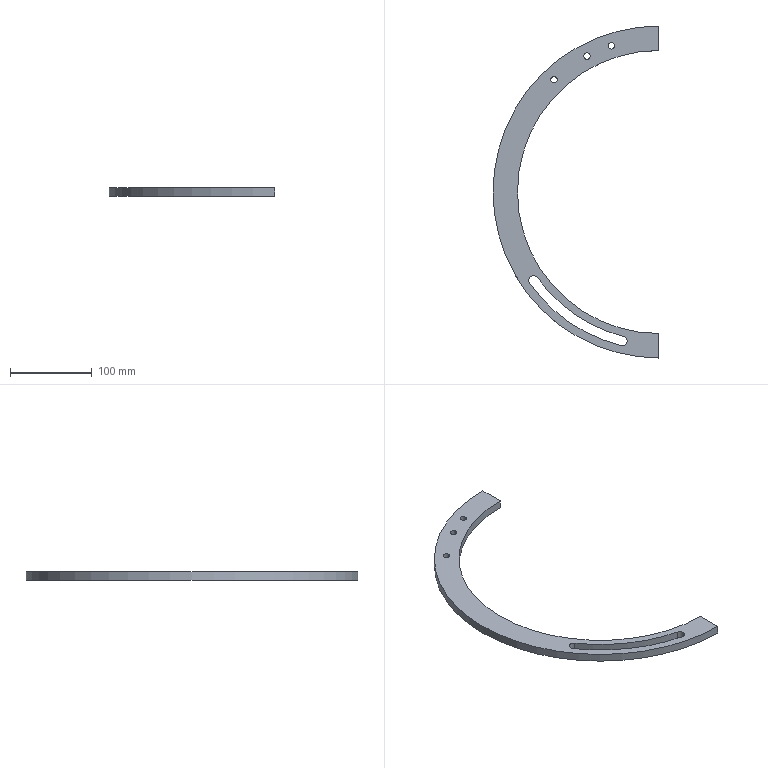Part | SolidWorks | features Cut 3, Extrusion 1 | 1 solid | 17 faces | box 203.295 x 406.59 x 10 mm | volume 159222 mm3 | cylinder 13 | plane 4 | commonest cylinder face diameters 8 x6 11.641 x3 346.59 x1 364.161 x1 387.442 x1 406.59 x1
STEP:
#1=CARTESIAN_POINT('',(166.898,320.188,0.));
#2=VERTEX_POINT('',#1);
#3=CARTESIAN_POINT('',(158.898,320.188,0.));
#4=VERTEX_POINT('',#3);
#5=CARTESIAN_POINT('',(162.898,320.188,0.));
#6=DIRECTION('',(0.,0.,-1.));
#7=DIRECTION('',(-1.,0.,0.));
#8=AXIS2_PLACEMENT_3D('',#5,#6,#7);
#9=CIRCLE('',#8,4.);
#10=EDGE_CURVE('',#2,#4,#9,.T.);
#11=ORIENTED_EDGE('',*,*,#10,.F.);
#12=CARTESIAN_POINT('',(166.898,320.188,-10.));
#13=VERTEX_POINT('',#12);
#14=CARTESIAN_POINT('',(166.898,320.188,0.));
#15=DIRECTION('',(0.,0.,-1.));
#16=VECTOR('',#15,1000.);
#17=LINE('',#14,#16);
#18=EDGE_CURVE('',#2,#13,#17,.T.);
#19=ORIENTED_EDGE('',*,*,#18,.T.);
#20=CARTESIAN_POINT('',(158.898,320.188,-10.));
#21=VERTEX_POINT('',#20);
#22=CARTESIAN_POINT('',(162.898,320.188,-10.));
#23=DIRECTION('',(0.,0.,1.));
#24=DIRECTION('',(1.,0.,0.));
#25=AXIS2_PLACEMENT_3D('',#22,#23,#24);
#26=CIRCLE('',#25,4.);
#27=EDGE_CURVE('',#21,#13,#26,.T.);
#28=ORIENTED_EDGE('',*,*,#27,.F.);
#29=CARTESIAN_POINT('',(158.898,320.188,0.));
#30=DIRECTION('',(0.,0.,-1.));
#31=VECTOR('',#30,1000.);
#32=LINE('',#29,#31);
#33=EDGE_CURVE('',#4,#21,#32,.T.);
#34=ORIENTED_EDGE('',*,*,#33,.F.);
#35=EDGE_LOOP('',(#11,#19,#28,#34));
#36=FACE_OUTER_BOUND('',#35,.T.);
#37=CARTESIAN_POINT('',(162.898,320.188,0.));
#38=DIRECTION('',(0.,0.,-1.));
#39=DIRECTION('',(-1.,0.,0.));
#40=AXIS2_PLACEMENT_3D('',#37,#38,#39);
#41=CYLINDRICAL_SURFACE('',#40,4.);
#42=ADVANCED_FACE('',(#36),#41,.F.);
#43=CARTESIAN_POINT('',(237.318,361.783,0.));
#44=VERTEX_POINT('',#43);
#45=CARTESIAN_POINT('',(229.318,361.783,0.));
#46=VERTEX_POINT('',#45);
#47=CARTESIAN_POINT('',(233.318,361.783,0.));
#48=DIRECTION('',(0.,0.,-1.));
#49=DIRECTION('',(-1.,0.,0.));
#50=AXIS2_PLACEMENT_3D('',#47,#48,#49);
#51=CIRCLE('',#50,4.);
#52=EDGE_CURVE('',#44,#46,#51,.T.);
#53=ORIENTED_EDGE('',*,*,#52,.F.);
#54=CARTESIAN_POINT('',(237.318,361.783,-10.));
#55=VERTEX_POINT('',#54);
#56=CARTESIAN_POINT('',(237.318,361.783,0.));
#57=DIRECTION('',(0.,0.,-1.));
#58=VECTOR('',#57,1000.);
#59=LINE('',#56,#58);
#60=EDGE_CURVE('',#44,#55,#59,.T.);
#61=ORIENTED_EDGE('',*,*,#60,.T.);
#62=CARTESIAN_POINT('',(229.318,361.783,-10.));
#63=VERTEX_POINT('',#62);
#64=CARTESIAN_POINT('',(233.318,361.783,-10.));
#65=DIRECTION('',(0.,0.,1.));
#66=DIRECTION('',(1.,0.,0.));
#67=AXIS2_PLACEMENT_3D('',#64,#65,#66);
#68=CIRCLE('',#67,4.);
#69=EDGE_CURVE('',#63,#55,#68,.T.);
#70=ORIENTED_EDGE('',*,*,#69,.F.);
#71=CARTESIAN_POINT('',(229.318,361.783,0.));
#72=DIRECTION('',(0.,0.,-1.));
#73=VECTOR('',#72,1000.);
#74=LINE('',#71,#73);
#75=EDGE_CURVE('',#46,#63,#74,.T.);
#76=ORIENTED_EDGE('',*,*,#75,.F.);
#77=EDGE_LOOP('',(#53,#61,#70,#76));
#78=FACE_OUTER_BOUND('',#77,.T.);
#79=CARTESIAN_POINT('',(233.318,361.783,0.));
#80=DIRECTION('',(0.,0.,-1.));
#81=DIRECTION('',(-1.,0.,0.));
#82=AXIS2_PLACEMENT_3D('',#79,#80,#81);
#83=CYLINDRICAL_SURFACE('',#82,4.);
#84=ADVANCED_FACE('',(#78),#83,.F.);
#85=CARTESIAN_POINT('',(207.412,349.105,0.));
#86=VERTEX_POINT('',#85);
#87=CARTESIAN_POINT('',(199.412,349.105,0.));
#88=VERTEX_POINT('',#87);
#89=CARTESIAN_POINT('',(203.412,349.105,0.));
#90=DIRECTION('',(0.,0.,-1.));
#91=DIRECTION('',(-1.,0.,0.));
#92=AXIS2_PLACEMENT_3D('',#89,#90,#91);
#93=CIRCLE('',#92,4.);
#94=EDGE_CURVE('',#86,#88,#93,.T.);
#95=ORIENTED_EDGE('',*,*,#94,.F.);
#96=CARTESIAN_POINT('',(207.412,349.105,-10.));
#97=VERTEX_POINT('',#96);
#98=CARTESIAN_POINT('',(207.412,349.105,0.));
#99=DIRECTION('',(0.,0.,-1.));
#100=VECTOR('',#99,1000.);
#101=LINE('',#98,#100);
#102=EDGE_CURVE('',#86,#97,#101,.T.);
#103=ORIENTED_EDGE('',*,*,#102,.T.);
#104=CARTESIAN_POINT('',(199.412,349.105,-10.));
#105=VERTEX_POINT('',#104);
#106=CARTESIAN_POINT('',(203.412,349.105,-10.));
#107=DIRECTION('',(0.,0.,1.));
#108=DIRECTION('',(1.,0.,0.));
#109=AXIS2_PLACEMENT_3D('',#106,#107,#108);
#110=CIRCLE('',#109,4.);
#111=EDGE_CURVE('',#105,#97,#110,.T.);
#112=ORIENTED_EDGE('',*,*,#111,.F.);
#113=CARTESIAN_POINT('',(199.412,349.105,0.));
#114=DIRECTION('',(0.,0.,-1.));
#115=VECTOR('',#114,1000.);
#116=LINE('',#113,#115);
#117=EDGE_CURVE('',#88,#105,#116,.T.);
#118=ORIENTED_EDGE('',*,*,#117,.F.);
#119=EDGE_LOOP('',(#95,#103,#112,#118));
#120=FACE_OUTER_BOUND('',#119,.T.);
#121=CARTESIAN_POINT('',(203.412,349.105,0.));
#122=DIRECTION('',(0.,0.,-1.));
#123=DIRECTION('',(-1.,0.,0.));
#124=AXIS2_PLACEMENT_3D('',#121,#122,#123);
#125=CYLINDRICAL_SURFACE('',#124,4.);
#126=ADVANCED_FACE('',(#120),#125,.F.);
#127=CARTESIAN_POINT('',(142.762,77.826,0.));
#128=VERTEX_POINT('',#127);
#129=CARTESIAN_POINT('',(132.185,74.473,0.));
#130=VERTEX_POINT('',#129);
#131=CARTESIAN_POINT('',(138.005,74.473,0.));
#132=DIRECTION('',(0.,0.,1.));
#133=DIRECTION('',(1.,0.,0.));
#134=AXIS2_PLACEMENT_3D('',#131,#132,#133);
#135=CIRCLE('',#134,5.82);
#136=EDGE_CURVE('',#128,#130,#135,.T.);
#137=ORIENTED_EDGE('',*,*,#136,.T.);
#138=CARTESIAN_POINT('',(132.185,74.473,-10.));
#139=VERTEX_POINT('',#138);
#140=CARTESIAN_POINT('',(132.185,74.473,175.));
#141=DIRECTION('',(0.,0.,-1.));
#142=VECTOR('',#141,1000.);
#143=LINE('',#140,#142);
#144=EDGE_CURVE('',#130,#139,#143,.T.);
#145=ORIENTED_EDGE('',*,*,#144,.T.);
#146=CARTESIAN_POINT('',(142.762,77.826,-10.));
#147=VERTEX_POINT('',#146);
#148=CARTESIAN_POINT('',(138.005,74.473,-10.));
#149=DIRECTION('',(0.,0.,-1.));
#150=DIRECTION('',(-1.,0.,0.));
#151=AXIS2_PLACEMENT_3D('',#148,#149,#150);
#152=CIRCLE('',#151,5.82);
#153=EDGE_CURVE('',#139,#147,#152,.T.);
#154=ORIENTED_EDGE('',*,*,#153,.T.);
#155=CARTESIAN_POINT('',(142.762,77.826,175.));
#156=DIRECTION('',(0.,0.,-1.));
#157=VECTOR('',#156,1000.);
#158=LINE('',#155,#157);
#159=EDGE_CURVE('',#128,#147,#158,.T.);
#160=ORIENTED_EDGE('',*,*,#159,.F.);
#161=EDGE_LOOP('',(#137,#145,#154,#160));
#162=FACE_OUTER_BOUND('',#161,.T.);
#163=CARTESIAN_POINT('',(138.005,74.473,175.));
#164=DIRECTION('',(0.,0.,-1.));
#165=DIRECTION('',(-1.,0.,0.));
#166=AXIS2_PLACEMENT_3D('',#163,#164,#165);
#167=CYLINDRICAL_SURFACE('',#166,5.82);
#168=ADVANCED_FACE('',(#162),#167,.F.);
#169=CARTESIAN_POINT('',(291.585,-20.564,0.));
#170=VERTEX_POINT('',#169);
#171=CARTESIAN_POINT('',(291.585,-20.564,-10.));
#172=VERTEX_POINT('',#171);
#173=CARTESIAN_POINT('',(291.585,-20.564,-10.));
#174=DIRECTION('',(0.,0.,-1.));
#175=VECTOR('',#174,1000.);
#176=LINE('',#173,#175);
#177=EDGE_CURVE('',#170,#172,#176,.T.);
#178=ORIENTED_EDGE('',*,*,#177,.F.);
#179=CARTESIAN_POINT('',(291.585,386.026,0.));
#180=VERTEX_POINT('',#179);
#181=CARTESIAN_POINT('',(291.585,182.731,0.));
#182=DIRECTION('',(0.,0.,1.));
#183=DIRECTION('',(1.,0.,0.));
#184=AXIS2_PLACEMENT_3D('',#181,#182,#183);
#185=CIRCLE('',#184,203.295);
#186=EDGE_CURVE('',#180,#170,#185,.T.);
#187=ORIENTED_EDGE('',*,*,#186,.F.);
#188=CARTESIAN_POINT('',(291.585,386.026,-10.));
#189=VERTEX_POINT('',#188);
#190=CARTESIAN_POINT('',(291.585,386.026,-10.));
#191=DIRECTION('',(0.,0.,1.));
#192=VECTOR('',#191,1000.);
#193=LINE('',#190,#192);
#194=EDGE_CURVE('',#189,#180,#193,.T.);
#195=ORIENTED_EDGE('',*,*,#194,.F.);
#196=CARTESIAN_POINT('',(291.585,182.731,-10.));
#197=DIRECTION('',(0.,0.,1.));
#198=DIRECTION('',(1.,0.,0.));
#199=AXIS2_PLACEMENT_3D('',#196,#197,#198);
#200=CIRCLE('',#199,203.295);
#201=EDGE_CURVE('',#189,#172,#200,.T.);
#202=ORIENTED_EDGE('',*,*,#201,.T.);
#203=EDGE_LOOP('',(#178,#187,#195,#202));
#204=FACE_OUTER_BOUND('',#203,.T.);
#205=CARTESIAN_POINT('',(291.585,182.731,-10.));
#206=DIRECTION('',(0.,0.,1.));
#207=DIRECTION('',(1.,0.,0.));
#208=AXIS2_PLACEMENT_3D('',#205,#206,#207);
#209=CYLINDRICAL_SURFACE('',#208,203.295);
#210=ADVANCED_FACE('',(#204),#209,.T.);
#211=ORIENTED_EDGE('',*,*,#27,.T.);
#212=CARTESIAN_POINT('',(162.898,320.188,-10.));
#213=DIRECTION('',(0.,0.,1.));
#214=DIRECTION('',(1.,0.,0.));
#215=AXIS2_PLACEMENT_3D('',#212,#213,#214);
#216=CIRCLE('',#215,4.);
#217=EDGE_CURVE('',#13,#21,#216,.T.);
#218=ORIENTED_EDGE('',*,*,#217,.T.);
#219=EDGE_LOOP('',(#211,#218));
#220=FACE_BOUND('',#219,.T.);
#221=ORIENTED_EDGE('',*,*,#69,.T.);
#222=CARTESIAN_POINT('',(233.318,361.783,-10.));
#223=DIRECTION('',(0.,0.,1.));
#224=DIRECTION('',(1.,0.,0.));
#225=AXIS2_PLACEMENT_3D('',#222,#223,#224);
#226=CIRCLE('',#225,4.);
#227=EDGE_CURVE('',#55,#63,#226,.T.);
#228=ORIENTED_EDGE('',*,*,#227,.T.);
#229=EDGE_LOOP('',(#221,#228));
#230=FACE_BOUND('',#229,.T.);
#231=ORIENTED_EDGE('',*,*,#111,.T.);
#232=CARTESIAN_POINT('',(203.412,349.105,-10.));
#233=DIRECTION('',(0.,0.,1.));
#234=DIRECTION('',(1.,0.,0.));
#235=AXIS2_PLACEMENT_3D('',#232,#233,#234);
#236=CIRCLE('',#235,4.);
#237=EDGE_CURVE('',#97,#105,#236,.T.);
#238=ORIENTED_EDGE('',*,*,#237,.T.);
#239=EDGE_LOOP('',(#231,#238));
#240=FACE_BOUND('',#239,.T.);
#241=CARTESIAN_POINT('',(245.463,-5.42,-10.));
#242=VERTEX_POINT('',#241);
#243=CARTESIAN_POINT('',(133.248,71.119,-10.));
#244=VERTEX_POINT('',#243);
#245=CARTESIAN_POINT('',(291.585,182.731,-10.));
#246=DIRECTION('',(0.,0.,-1.));
#247=DIRECTION('',(-1.,0.,0.));
#248=AXIS2_PLACEMENT_3D('',#245,#246,#247);
#249=CIRCLE('',#248,193.721);
#250=EDGE_CURVE('',#242,#244,#249,.T.);
#251=ORIENTED_EDGE('',*,*,#250,.F.);
#252=CARTESIAN_POINT('',(248.235,5.886,-10.));
#253=VERTEX_POINT('',#252);
#254=CARTESIAN_POINT('',(246.849,0.2333,-10.));
#255=DIRECTION('',(0.,0.,-1.));
#256=DIRECTION('',(-1.,0.,0.));
#257=AXIS2_PLACEMENT_3D('',#254,#255,#256);
#258=CIRCLE('',#257,5.82);
#259=EDGE_CURVE('',#253,#242,#258,.T.);
#260=ORIENTED_EDGE('',*,*,#259,.F.);
#261=CARTESIAN_POINT('',(291.585,182.731,-10.));
#262=DIRECTION('',(0.,0.,1.));
#263=DIRECTION('',(-1.,0.,0.));
#264=AXIS2_PLACEMENT_3D('',#261,#262,#263);
#265=CIRCLE('',#264,182.08);
#266=EDGE_CURVE('',#147,#253,#265,.T.);
#267=ORIENTED_EDGE('',*,*,#266,.F.);
#268=ORIENTED_EDGE('',*,*,#153,.F.);
#269=CARTESIAN_POINT('',(138.005,74.473,-10.));
#270=DIRECTION('',(0.,0.,-1.));
#271=DIRECTION('',(-1.,0.,0.));
#272=AXIS2_PLACEMENT_3D('',#269,#270,#271);
#273=CIRCLE('',#272,5.82);
#274=EDGE_CURVE('',#244,#139,#273,.T.);
#275=ORIENTED_EDGE('',*,*,#274,.F.);
#276=EDGE_LOOP('',(#251,#260,#267,#268,#275));
#277=FACE_BOUND('',#276,.T.);
#278=CARTESIAN_POINT('',(291.585,356.026,-10.));
#279=VERTEX_POINT('',#278);
#280=CARTESIAN_POINT('',(291.585,9.436,-10.));
#281=VERTEX_POINT('',#280);
#282=CARTESIAN_POINT('',(291.585,182.731,-10.));
#283=DIRECTION('',(0.,0.,1.));
#284=DIRECTION('',(1.,0.,0.));
#285=AXIS2_PLACEMENT_3D('',#282,#283,#284);
#286=CIRCLE('',#285,173.295);
#287=EDGE_CURVE('',#279,#281,#286,.T.);
#288=ORIENTED_EDGE('',*,*,#287,.T.);
#289=CARTESIAN_POINT('',(291.585,9.436,-10.));
#290=DIRECTION('',(0.,1.,0.));
#291=VECTOR('',#290,1000.);
#292=LINE('',#289,#291);
#293=EDGE_CURVE('',#172,#281,#292,.T.);
#294=ORIENTED_EDGE('',*,*,#293,.F.);
#295=ORIENTED_EDGE('',*,*,#201,.F.);
#296=CARTESIAN_POINT('',(291.585,356.026,-10.));
#297=DIRECTION('',(0.,1.,0.));
#298=VECTOR('',#297,1000.);
#299=LINE('',#296,#298);
#300=EDGE_CURVE('',#279,#189,#299,.T.);
#301=ORIENTED_EDGE('',*,*,#300,.F.);
#302=EDGE_LOOP('',(#288,#294,#295,#301));
#303=FACE_OUTER_BOUND('',#302,.T.);
#304=CARTESIAN_POINT('',(291.585,182.731,-10.));
#305=DIRECTION('',(0.,0.,1.));
#306=DIRECTION('',(1.,0.,0.));
#307=AXIS2_PLACEMENT_3D('',#304,#305,#306);
#308=PLANE('',#307);
#309=ADVANCED_FACE('',(#220,#230,#240,#277,#303),#308,.F.);
#310=CARTESIAN_POINT('',(162.898,320.188,0.));
#311=DIRECTION('',(0.,0.,-1.));
#312=DIRECTION('',(-1.,0.,0.));
#313=AXIS2_PLACEMENT_3D('',#310,#311,#312);
#314=CIRCLE('',#313,4.);
#315=EDGE_CURVE('',#4,#2,#314,.T.);
#316=ORIENTED_EDGE('',*,*,#315,.T.);
#317=ORIENTED_EDGE('',*,*,#10,.T.);
#318=EDGE_LOOP('',(#316,#317));
#319=FACE_BOUND('',#318,.T.);
#320=CARTESIAN_POINT('',(233.318,361.783,0.));
#321=DIRECTION('',(0.,0.,-1.));
#322=DIRECTION('',(-1.,0.,0.));
#323=AXIS2_PLACEMENT_3D('',#320,#321,#322);
#324=CIRCLE('',#323,4.);
#325=EDGE_CURVE('',#46,#44,#324,.T.);
#326=ORIENTED_EDGE('',*,*,#325,.T.);
#327=ORIENTED_EDGE('',*,*,#52,.T.);
#328=EDGE_LOOP('',(#326,#327));
#329=FACE_BOUND('',#328,.T.);
#330=CARTESIAN_POINT('',(203.412,349.105,0.));
#331=DIRECTION('',(0.,0.,-1.));
#332=DIRECTION('',(-1.,0.,0.));
#333=AXIS2_PLACEMENT_3D('',#330,#331,#332);
#334=CIRCLE('',#333,4.);
#335=EDGE_CURVE('',#88,#86,#334,.T.);
#336=ORIENTED_EDGE('',*,*,#335,.T.);
#337=ORIENTED_EDGE('',*,*,#94,.T.);
#338=EDGE_LOOP('',(#336,#337));
#339=FACE_BOUND('',#338,.T.);
#340=CARTESIAN_POINT('',(245.463,-5.42,0.));
#341=VERTEX_POINT('',#340);
#342=CARTESIAN_POINT('',(248.235,5.886,0.));
#343=VERTEX_POINT('',#342);
#344=CARTESIAN_POINT('',(246.849,0.2333,0.));
#345=DIRECTION('',(0.,0.,1.));
#346=DIRECTION('',(1.,0.,0.));
#347=AXIS2_PLACEMENT_3D('',#344,#345,#346);
#348=CIRCLE('',#347,5.82);
#349=EDGE_CURVE('',#341,#343,#348,.T.);
#350=ORIENTED_EDGE('',*,*,#349,.F.);
#351=CARTESIAN_POINT('',(133.248,71.119,0.));
#352=VERTEX_POINT('',#351);
#353=CARTESIAN_POINT('',(291.585,182.731,0.));
#354=DIRECTION('',(0.,0.,1.));
#355=DIRECTION('',(1.,0.,0.));
#356=AXIS2_PLACEMENT_3D('',#353,#354,#355);
#357=CIRCLE('',#356,193.721);
#358=EDGE_CURVE('',#352,#341,#357,.T.);
#359=ORIENTED_EDGE('',*,*,#358,.F.);
#360=CARTESIAN_POINT('',(138.005,74.473,0.));
#361=DIRECTION('',(0.,0.,1.));
#362=DIRECTION('',(1.,0.,0.));
#363=AXIS2_PLACEMENT_3D('',#360,#361,#362);
#364=CIRCLE('',#363,5.82);
#365=EDGE_CURVE('',#130,#352,#364,.T.);
#366=ORIENTED_EDGE('',*,*,#365,.F.);
#367=ORIENTED_EDGE('',*,*,#136,.F.);
#368=CARTESIAN_POINT('',(291.585,182.731,0.));
#369=DIRECTION('',(0.,0.,-1.));
#370=DIRECTION('',(1.,0.,0.));
#371=AXIS2_PLACEMENT_3D('',#368,#369,#370);
#372=CIRCLE('',#371,182.08);
#373=EDGE_CURVE('',#343,#128,#372,.T.);
#374=ORIENTED_EDGE('',*,*,#373,.F.);
#375=EDGE_LOOP('',(#350,#359,#366,#367,#374));
#376=FACE_BOUND('',#375,.T.);
#377=CARTESIAN_POINT('',(291.585,9.436,0.));
#378=VERTEX_POINT('',#377);
#379=CARTESIAN_POINT('',(291.585,182.731,0.));
#380=DIRECTION('',(0.,-1.,0.));
#381=VECTOR('',#380,1000.);
#382=LINE('',#379,#381);
#383=EDGE_CURVE('',#378,#170,#382,.T.);
#384=ORIENTED_EDGE('',*,*,#383,.F.);
#385=CARTESIAN_POINT('',(291.585,356.026,0.));
#386=VERTEX_POINT('',#385);
#387=CARTESIAN_POINT('',(291.585,182.731,0.));
#388=DIRECTION('',(0.,0.,1.));
#389=DIRECTION('',(1.,0.,0.));
#390=AXIS2_PLACEMENT_3D('',#387,#388,#389);
#391=CIRCLE('',#390,173.295);
#392=EDGE_CURVE('',#386,#378,#391,.T.);
#393=ORIENTED_EDGE('',*,*,#392,.F.);
#394=CARTESIAN_POINT('',(291.585,182.731,0.));
#395=DIRECTION('',(0.,-1.,0.));
#396=VECTOR('',#395,1000.);
#397=LINE('',#394,#396);
#398=EDGE_CURVE('',#180,#386,#397,.T.);
#399=ORIENTED_EDGE('',*,*,#398,.F.);
#400=ORIENTED_EDGE('',*,*,#186,.T.);
#401=EDGE_LOOP('',(#384,#393,#399,#400));
#402=FACE_OUTER_BOUND('',#401,.T.);
#403=CARTESIAN_POINT('',(291.585,182.731,0.));
#404=DIRECTION('',(0.,0.,1.));
#405=DIRECTION('',(1.,0.,0.));
#406=AXIS2_PLACEMENT_3D('',#403,#404,#405);
#407=PLANE('',#406);
#408=ADVANCED_FACE('',(#319,#329,#339,#376,#402),#407,.T.);
#409=ORIENTED_EDGE('',*,*,#392,.T.);
#410=CARTESIAN_POINT('',(291.585,9.436,-10.));
#411=DIRECTION('',(0.,0.,-1.));
#412=VECTOR('',#411,1000.);
#413=LINE('',#410,#412);
#414=EDGE_CURVE('',#378,#281,#413,.T.);
#415=ORIENTED_EDGE('',*,*,#414,.T.);
#416=ORIENTED_EDGE('',*,*,#287,.F.);
#417=CARTESIAN_POINT('',(291.585,356.026,-10.));
#418=DIRECTION('',(0.,0.,1.));
#419=VECTOR('',#418,1000.);
#420=LINE('',#417,#419);
#421=EDGE_CURVE('',#279,#386,#420,.T.);
#422=ORIENTED_EDGE('',*,*,#421,.T.);
#423=EDGE_LOOP('',(#409,#415,#416,#422));
#424=FACE_OUTER_BOUND('',#423,.T.);
#425=CARTESIAN_POINT('',(291.585,182.731,-10.));
#426=DIRECTION('',(0.,0.,1.));
#427=DIRECTION('',(1.,0.,0.));
#428=AXIS2_PLACEMENT_3D('',#425,#426,#427);
#429=CYLINDRICAL_SURFACE('',#428,173.295);
#430=ADVANCED_FACE('',(#424),#429,.F.);
#431=ORIENTED_EDGE('',*,*,#194,.T.);
#432=ORIENTED_EDGE('',*,*,#398,.T.);
#433=ORIENTED_EDGE('',*,*,#421,.F.);
#434=ORIENTED_EDGE('',*,*,#300,.T.);
#435=EDGE_LOOP('',(#431,#432,#433,#434));
#436=FACE_OUTER_BOUND('',#435,.T.);
#437=CARTESIAN_POINT('',(291.585,356.026,175.));
#438=DIRECTION('',(-1.,0.,0.));
#439=DIRECTION('',(0.,0.,1.));
#440=AXIS2_PLACEMENT_3D('',#437,#438,#439);
#441=PLANE('',#440);
#442=ADVANCED_FACE('',(#436),#441,.F.);
#443=ORIENTED_EDGE('',*,*,#177,.T.);
#444=ORIENTED_EDGE('',*,*,#293,.T.);
#445=ORIENTED_EDGE('',*,*,#414,.F.);
#446=ORIENTED_EDGE('',*,*,#383,.T.);
#447=EDGE_LOOP('',(#443,#444,#445,#446));
#448=FACE_OUTER_BOUND('',#447,.T.);
#449=CARTESIAN_POINT('',(291.585,9.436,175.));
#450=DIRECTION('',(-1.,0.,0.));
#451=DIRECTION('',(0.,0.,1.));
#452=AXIS2_PLACEMENT_3D('',#449,#450,#451);
#453=PLANE('',#452);
#454=ADVANCED_FACE('',(#448),#453,.F.);
#455=ORIENTED_EDGE('',*,*,#349,.T.);
#456=CARTESIAN_POINT('',(248.235,5.886,175.));
#457=DIRECTION('',(0.,0.,-1.));
#458=VECTOR('',#457,1000.);
#459=LINE('',#456,#458);
#460=EDGE_CURVE('',#343,#253,#459,.T.);
#461=ORIENTED_EDGE('',*,*,#460,.T.);
#462=ORIENTED_EDGE('',*,*,#259,.T.);
#463=CARTESIAN_POINT('',(245.463,-5.42,175.));
#464=DIRECTION('',(0.,0.,-1.));
#465=VECTOR('',#464,1000.);
#466=LINE('',#463,#465);
#467=EDGE_CURVE('',#341,#242,#466,.T.);
#468=ORIENTED_EDGE('',*,*,#467,.F.);
#469=EDGE_LOOP('',(#455,#461,#462,#468));
#470=FACE_OUTER_BOUND('',#469,.T.);
#471=CARTESIAN_POINT('',(246.849,0.2333,175.));
#472=DIRECTION('',(0.,0.,-1.));
#473=DIRECTION('',(-1.,0.,0.));
#474=AXIS2_PLACEMENT_3D('',#471,#472,#473);
#475=CYLINDRICAL_SURFACE('',#474,5.82);
#476=ADVANCED_FACE('',(#470),#475,.F.);
#477=ORIENTED_EDGE('',*,*,#373,.T.);
#478=ORIENTED_EDGE('',*,*,#159,.T.);
#479=ORIENTED_EDGE('',*,*,#266,.T.);
#480=ORIENTED_EDGE('',*,*,#460,.F.);
#481=EDGE_LOOP('',(#477,#478,#479,#480));
#482=FACE_OUTER_BOUND('',#481,.T.);
#483=CARTESIAN_POINT('',(291.585,182.731,175.));
#484=DIRECTION('',(0.,0.,-1.));
#485=DIRECTION('',(-1.,0.,0.));
#486=AXIS2_PLACEMENT_3D('',#483,#484,#485);
#487=CYLINDRICAL_SURFACE('',#486,182.08);
#488=ADVANCED_FACE('',(#482),#487,.T.);
#489=ORIENTED_EDGE('',*,*,#144,.F.);
#490=ORIENTED_EDGE('',*,*,#365,.T.);
#491=CARTESIAN_POINT('',(133.248,71.119,175.));
#492=DIRECTION('',(0.,0.,-1.));
#493=VECTOR('',#492,1000.);
#494=LINE('',#491,#493);
#495=EDGE_CURVE('',#352,#244,#494,.T.);
#496=ORIENTED_EDGE('',*,*,#495,.T.);
#497=ORIENTED_EDGE('',*,*,#274,.T.);
#498=EDGE_LOOP('',(#489,#490,#496,#497));
#499=FACE_OUTER_BOUND('',#498,.T.);
#500=CARTESIAN_POINT('',(138.005,74.473,175.));
#501=DIRECTION('',(0.,0.,-1.));
#502=DIRECTION('',(-1.,0.,0.));
#503=AXIS2_PLACEMENT_3D('',#500,#501,#502);
#504=CYLINDRICAL_SURFACE('',#503,5.82);
#505=ADVANCED_FACE('',(#499),#504,.F.);
#506=ORIENTED_EDGE('',*,*,#358,.T.);
#507=ORIENTED_EDGE('',*,*,#467,.T.);
#508=ORIENTED_EDGE('',*,*,#250,.T.);
#509=ORIENTED_EDGE('',*,*,#495,.F.);
#510=EDGE_LOOP('',(#506,#507,#508,#509));
#511=FACE_OUTER_BOUND('',#510,.T.);
#512=CARTESIAN_POINT('',(291.585,182.731,175.));
#513=DIRECTION('',(0.,0.,-1.));
#514=DIRECTION('',(-1.,0.,0.));
#515=AXIS2_PLACEMENT_3D('',#512,#513,#514);
#516=CYLINDRICAL_SURFACE('',#515,193.721);
#517=ADVANCED_FACE('',(#511),#516,.F.);
#518=ORIENTED_EDGE('',*,*,#102,.F.);
#519=ORIENTED_EDGE('',*,*,#335,.F.);
#520=ORIENTED_EDGE('',*,*,#117,.T.);
#521=ORIENTED_EDGE('',*,*,#237,.F.);
#522=EDGE_LOOP('',(#518,#519,#520,#521));
#523=FACE_OUTER_BOUND('',#522,.T.);
#524=CARTESIAN_POINT('',(203.412,349.105,0.));
#525=DIRECTION('',(0.,0.,-1.));
#526=DIRECTION('',(-1.,0.,0.));
#527=AXIS2_PLACEMENT_3D('',#524,#525,#526);
#528=CYLINDRICAL_SURFACE('',#527,4.);
#529=ADVANCED_FACE('',(#523),#528,.F.);
#530=ORIENTED_EDGE('',*,*,#60,.F.);
#531=ORIENTED_EDGE('',*,*,#325,.F.);
#532=ORIENTED_EDGE('',*,*,#75,.T.);
#533=ORIENTED_EDGE('',*,*,#227,.F.);
#534=EDGE_LOOP('',(#530,#531,#532,#533));
#535=FACE_OUTER_BOUND('',#534,.T.);
#536=CARTESIAN_POINT('',(233.318,361.783,0.));
#537=DIRECTION('',(0.,0.,-1.));
#538=DIRECTION('',(-1.,0.,0.));
#539=AXIS2_PLACEMENT_3D('',#536,#537,#538);
#540=CYLINDRICAL_SURFACE('',#539,4.);
#541=ADVANCED_FACE('',(#535),#540,.F.);
#542=ORIENTED_EDGE('',*,*,#18,.F.);
#543=ORIENTED_EDGE('',*,*,#315,.F.);
#544=ORIENTED_EDGE('',*,*,#33,.T.);
#545=ORIENTED_EDGE('',*,*,#217,.F.);
#546=EDGE_LOOP('',(#542,#543,#544,#545));
#547=FACE_OUTER_BOUND('',#546,.T.);
#548=CARTESIAN_POINT('',(162.898,320.188,0.));
#549=DIRECTION('',(0.,0.,-1.));
#550=DIRECTION('',(-1.,0.,0.));
#551=AXIS2_PLACEMENT_3D('',#548,#549,#550);
#552=CYLINDRICAL_SURFACE('',#551,4.);
#553=ADVANCED_FACE('',(#547),#552,.F.);
#554=CLOSED_SHELL('',(#42,#84,#126,#168,#210,#309,#408,#430,#442,#454,#476,#488,#505,#517,#529,#541,#553));
#555=MANIFOLD_SOLID_BREP('',#554);
#556=CARTESIAN_POINT('',(0.,0.,0.));
#557=DIRECTION('',(0.,0.,1.));
#558=DIRECTION('',(1.,0.,0.));
#559=AXIS2_PLACEMENT_3D('',#556,#557,#558);
#560=(LENGTH_UNIT()NAMED_UNIT(*)SI_UNIT(.MILLI.,.METRE.));
#561=UNCERTAINTY_MEASURE_WITH_UNIT(LENGTH_MEASURE(0.00001),#560,'','');
#562=(NAMED_UNIT(*)PLANE_ANGLE_UNIT()SI_UNIT($,.RADIAN.));
#563=(NAMED_UNIT(*)SI_UNIT($,.STERADIAN.)SOLID_ANGLE_UNIT());
#564=(GEOMETRIC_REPRESENTATION_CONTEXT(3)GLOBAL_UNCERTAINTY_ASSIGNED_CONTEXT((#561))GLOBAL_UNIT_ASSIGNED_CONTEXT((#560,#562,#563))REPRESENTATION_CONTEXT('',''));
#565=ADVANCED_BREP_SHAPE_REPRESENTATION('',(#555,#559),#564);